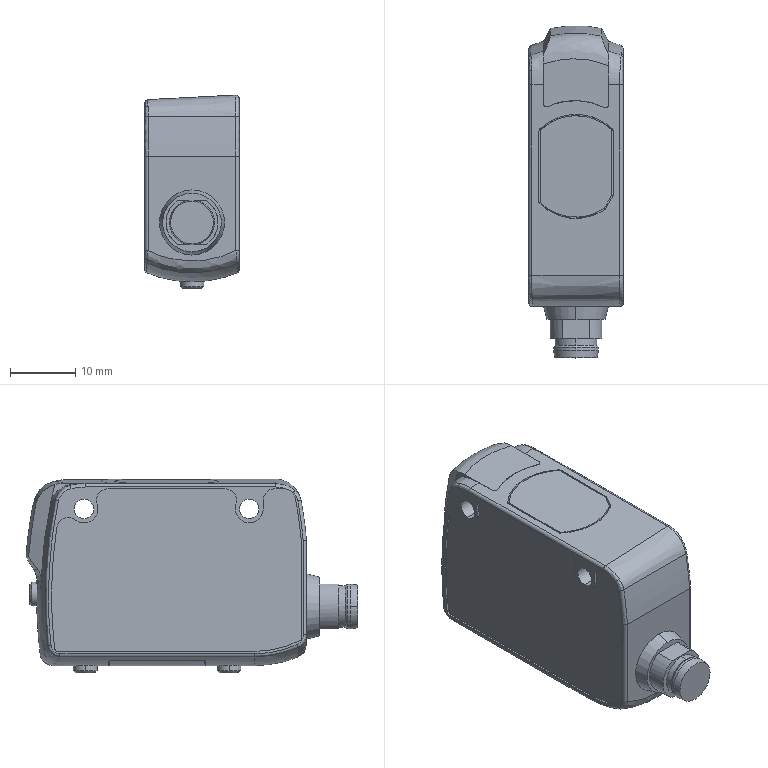Part | STEP file | LR-ZH500CP-Part-1-3 | 1 solid | 175 faces | box 14.5 x 51.056 x 29.773 mm | volume 15982 mm3 | cylinder 81 | plane 48 | spline 34 | cone 12 | commonest cylinder face diameters 1 x22 3.6 x11 0.6 x9 3.64 x6 4.3 x6 3 x4